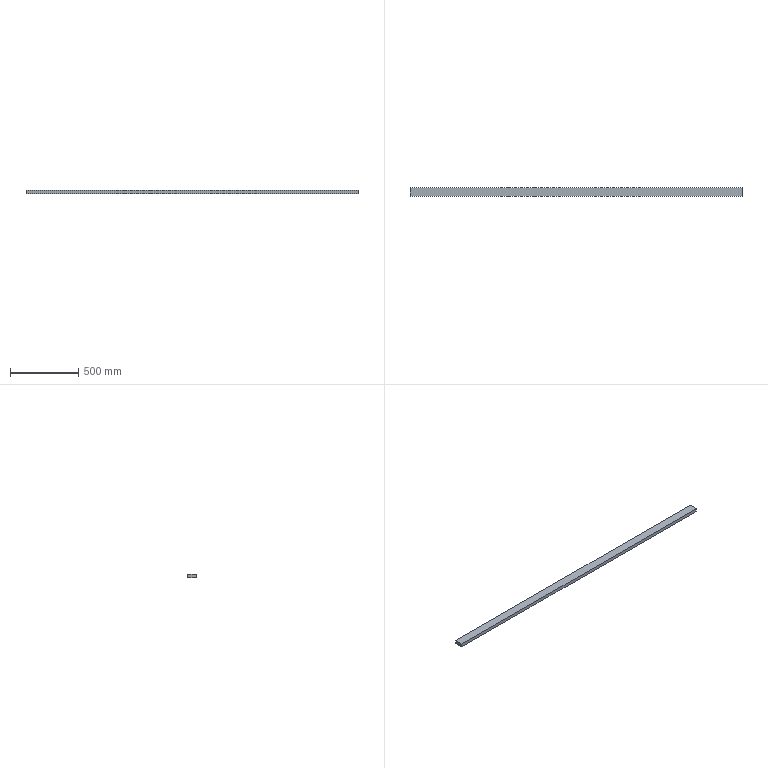Part | SolidWorks | features Extrusion 1 | 1 solid | 6 faces | box 2425 x 63 x 25 mm | volume 3819375 mm3 | plane 6
STEP:
#1=CARTESIAN_POINT('',(0.,63.,0.));
#2=VERTEX_POINT('',#1);
#3=CARTESIAN_POINT('',(0.,0.,0.));
#4=VERTEX_POINT('',#3);
#5=CARTESIAN_POINT('',(0.,0.,0.));
#6=DIRECTION('',(0.,-1.,0.));
#7=VECTOR('',#6,1000.);
#8=LINE('',#5,#7);
#9=EDGE_CURVE('',#2,#4,#8,.T.);
#10=ORIENTED_EDGE('',*,*,#9,.T.);
#11=CARTESIAN_POINT('',(0.,0.,25.));
#12=VERTEX_POINT('',#11);
#13=CARTESIAN_POINT('',(0.,0.,25.));
#14=DIRECTION('',(0.,0.,-1.));
#15=VECTOR('',#14,1000.);
#16=LINE('',#13,#15);
#17=EDGE_CURVE('',#12,#4,#16,.T.);
#18=ORIENTED_EDGE('',*,*,#17,.F.);
#19=CARTESIAN_POINT('',(0.,63.,25.));
#20=VERTEX_POINT('',#19);
#21=CARTESIAN_POINT('',(0.,0.,25.));
#22=DIRECTION('',(0.,-1.,0.));
#23=VECTOR('',#22,1000.);
#24=LINE('',#21,#23);
#25=EDGE_CURVE('',#20,#12,#24,.T.);
#26=ORIENTED_EDGE('',*,*,#25,.F.);
#27=CARTESIAN_POINT('',(0.,63.,25.));
#28=DIRECTION('',(0.,0.,-1.));
#29=VECTOR('',#28,1000.);
#30=LINE('',#27,#29);
#31=EDGE_CURVE('',#20,#2,#30,.T.);
#32=ORIENTED_EDGE('',*,*,#31,.T.);
#33=EDGE_LOOP('',(#10,#18,#26,#32));
#34=FACE_OUTER_BOUND('',#33,.T.);
#35=CARTESIAN_POINT('',(0.,0.,25.));
#36=DIRECTION('',(1.,0.,0.));
#37=DIRECTION('',(0.,0.,-1.));
#38=AXIS2_PLACEMENT_3D('',#35,#36,#37);
#39=PLANE('',#38);
#40=ADVANCED_FACE('',(#34),#39,.F.);
#41=CARTESIAN_POINT('',(2425.,0.,0.));
#42=VERTEX_POINT('',#41);
#43=CARTESIAN_POINT('',(0.,0.,0.));
#44=DIRECTION('',(1.,0.,0.));
#45=VECTOR('',#44,1000.);
#46=LINE('',#43,#45);
#47=EDGE_CURVE('',#4,#42,#46,.T.);
#48=ORIENTED_EDGE('',*,*,#47,.T.);
#49=CARTESIAN_POINT('',(2425.,0.,25.));
#50=VERTEX_POINT('',#49);
#51=CARTESIAN_POINT('',(2425.,0.,25.));
#52=DIRECTION('',(0.,0.,-1.));
#53=VECTOR('',#52,1000.);
#54=LINE('',#51,#53);
#55=EDGE_CURVE('',#50,#42,#54,.T.);
#56=ORIENTED_EDGE('',*,*,#55,.F.);
#57=CARTESIAN_POINT('',(0.,0.,25.));
#58=DIRECTION('',(1.,0.,0.));
#59=VECTOR('',#58,1000.);
#60=LINE('',#57,#59);
#61=EDGE_CURVE('',#12,#50,#60,.T.);
#62=ORIENTED_EDGE('',*,*,#61,.F.);
#63=ORIENTED_EDGE('',*,*,#17,.T.);
#64=EDGE_LOOP('',(#48,#56,#62,#63));
#65=FACE_OUTER_BOUND('',#64,.T.);
#66=CARTESIAN_POINT('',(0.,0.,25.));
#67=DIRECTION('',(0.,1.,0.));
#68=DIRECTION('',(0.,0.,1.));
#69=AXIS2_PLACEMENT_3D('',#66,#67,#68);
#70=PLANE('',#69);
#71=ADVANCED_FACE('',(#65),#70,.F.);
#72=CARTESIAN_POINT('',(2425.,63.,0.));
#73=VERTEX_POINT('',#72);
#74=CARTESIAN_POINT('',(2425.,0.,0.));
#75=DIRECTION('',(0.,1.,0.));
#76=VECTOR('',#75,1000.);
#77=LINE('',#74,#76);
#78=EDGE_CURVE('',#42,#73,#77,.T.);
#79=ORIENTED_EDGE('',*,*,#78,.T.);
#80=CARTESIAN_POINT('',(2425.,63.,25.));
#81=VERTEX_POINT('',#80);
#82=CARTESIAN_POINT('',(2425.,63.,25.));
#83=DIRECTION('',(0.,0.,-1.));
#84=VECTOR('',#83,1000.);
#85=LINE('',#82,#84);
#86=EDGE_CURVE('',#81,#73,#85,.T.);
#87=ORIENTED_EDGE('',*,*,#86,.F.);
#88=CARTESIAN_POINT('',(2425.,0.,25.));
#89=DIRECTION('',(0.,1.,0.));
#90=VECTOR('',#89,1000.);
#91=LINE('',#88,#90);
#92=EDGE_CURVE('',#50,#81,#91,.T.);
#93=ORIENTED_EDGE('',*,*,#92,.F.);
#94=ORIENTED_EDGE('',*,*,#55,.T.);
#95=EDGE_LOOP('',(#79,#87,#93,#94));
#96=FACE_OUTER_BOUND('',#95,.T.);
#97=CARTESIAN_POINT('',(2425.,0.,25.));
#98=DIRECTION('',(-1.,0.,0.));
#99=DIRECTION('',(0.,0.,1.));
#100=AXIS2_PLACEMENT_3D('',#97,#98,#99);
#101=PLANE('',#100);
#102=ADVANCED_FACE('',(#96),#101,.F.);
#103=CARTESIAN_POINT('',(0.,63.,0.));
#104=DIRECTION('',(-1.,0.,0.));
#105=VECTOR('',#104,1000.);
#106=LINE('',#103,#105);
#107=EDGE_CURVE('',#73,#2,#106,.T.);
#108=ORIENTED_EDGE('',*,*,#107,.T.);
#109=ORIENTED_EDGE('',*,*,#31,.F.);
#110=CARTESIAN_POINT('',(0.,63.,25.));
#111=DIRECTION('',(-1.,0.,0.));
#112=VECTOR('',#111,1000.);
#113=LINE('',#110,#112);
#114=EDGE_CURVE('',#81,#20,#113,.T.);
#115=ORIENTED_EDGE('',*,*,#114,.F.);
#116=ORIENTED_EDGE('',*,*,#86,.T.);
#117=EDGE_LOOP('',(#108,#109,#115,#116));
#118=FACE_OUTER_BOUND('',#117,.T.);
#119=CARTESIAN_POINT('',(0.,63.,25.));
#120=DIRECTION('',(0.,-1.,0.));
#121=DIRECTION('',(0.,0.,-1.));
#122=AXIS2_PLACEMENT_3D('',#119,#120,#121);
#123=PLANE('',#122);
#124=ADVANCED_FACE('',(#118),#123,.F.);
#125=ORIENTED_EDGE('',*,*,#25,.T.);
#126=ORIENTED_EDGE('',*,*,#61,.T.);
#127=ORIENTED_EDGE('',*,*,#92,.T.);
#128=ORIENTED_EDGE('',*,*,#114,.T.);
#129=EDGE_LOOP('',(#125,#126,#127,#128));
#130=FACE_OUTER_BOUND('',#129,.T.);
#131=CARTESIAN_POINT('',(0.,63.,25.));
#132=DIRECTION('',(0.,0.,-1.));
#133=DIRECTION('',(-1.,0.,0.));
#134=AXIS2_PLACEMENT_3D('',#131,#132,#133);
#135=PLANE('',#134);
#136=ADVANCED_FACE('',(#130),#135,.F.);
#137=ORIENTED_EDGE('',*,*,#9,.F.);
#138=ORIENTED_EDGE('',*,*,#107,.F.);
#139=ORIENTED_EDGE('',*,*,#78,.F.);
#140=ORIENTED_EDGE('',*,*,#47,.F.);
#141=EDGE_LOOP('',(#137,#138,#139,#140));
#142=FACE_OUTER_BOUND('',#141,.T.);
#143=CARTESIAN_POINT('',(0.,63.,0.));
#144=DIRECTION('',(0.,0.,-1.));
#145=DIRECTION('',(-1.,0.,0.));
#146=AXIS2_PLACEMENT_3D('',#143,#144,#145);
#147=PLANE('',#146);
#148=ADVANCED_FACE('',(#142),#147,.T.);
#149=CLOSED_SHELL('',(#40,#71,#102,#124,#136,#148));
#150=MANIFOLD_SOLID_BREP('',#149);
#151=CARTESIAN_POINT('',(0.,0.,0.));
#152=DIRECTION('',(0.,0.,1.));
#153=DIRECTION('',(1.,0.,0.));
#154=AXIS2_PLACEMENT_3D('',#151,#152,#153);
#155=(LENGTH_UNIT()NAMED_UNIT(*)SI_UNIT(.MILLI.,.METRE.));
#156=UNCERTAINTY_MEASURE_WITH_UNIT(LENGTH_MEASURE(0.00001),#155,'','');
#157=(NAMED_UNIT(*)PLANE_ANGLE_UNIT()SI_UNIT($,.RADIAN.));
#158=(NAMED_UNIT(*)SI_UNIT($,.STERADIAN.)SOLID_ANGLE_UNIT());
#159=(GEOMETRIC_REPRESENTATION_CONTEXT(3)GLOBAL_UNCERTAINTY_ASSIGNED_CONTEXT((#156))GLOBAL_UNIT_ASSIGNED_CONTEXT((#155,#157,#158))REPRESENTATION_CONTEXT('',''));
#160=ADVANCED_BREP_SHAPE_REPRESENTATION('',(#150,#154),#159);